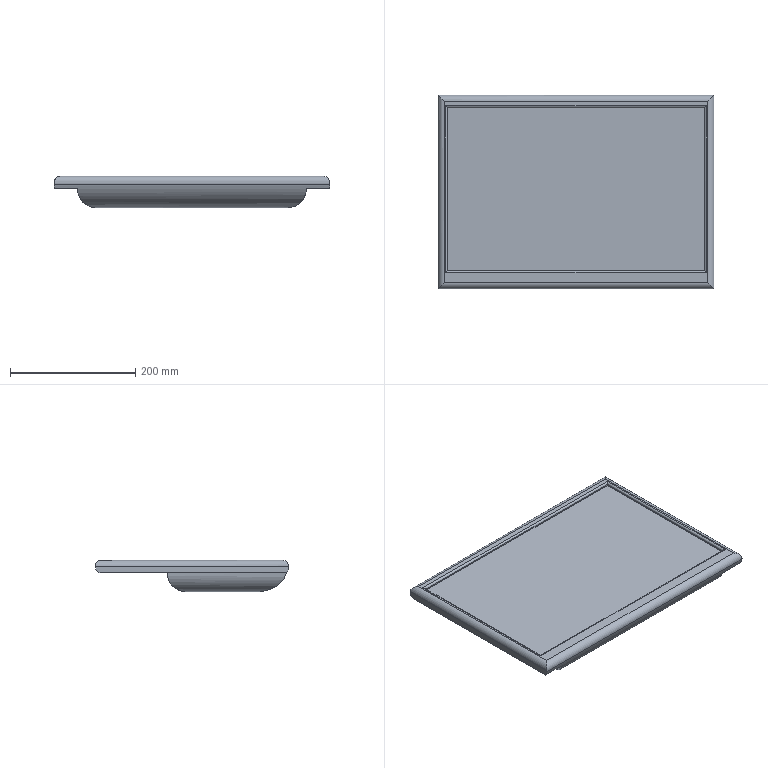Part | STEP file | computer monitor | 1 solid | 32 faces | box 440 x 308.73 x 50 mm | volume 3953854 mm3 | cylinder 17 | plane 11 | cone 4 | commonest cylinder face diameters 3.3 x4 6 x4 20 x4 60 x3 5 x1 100 x1